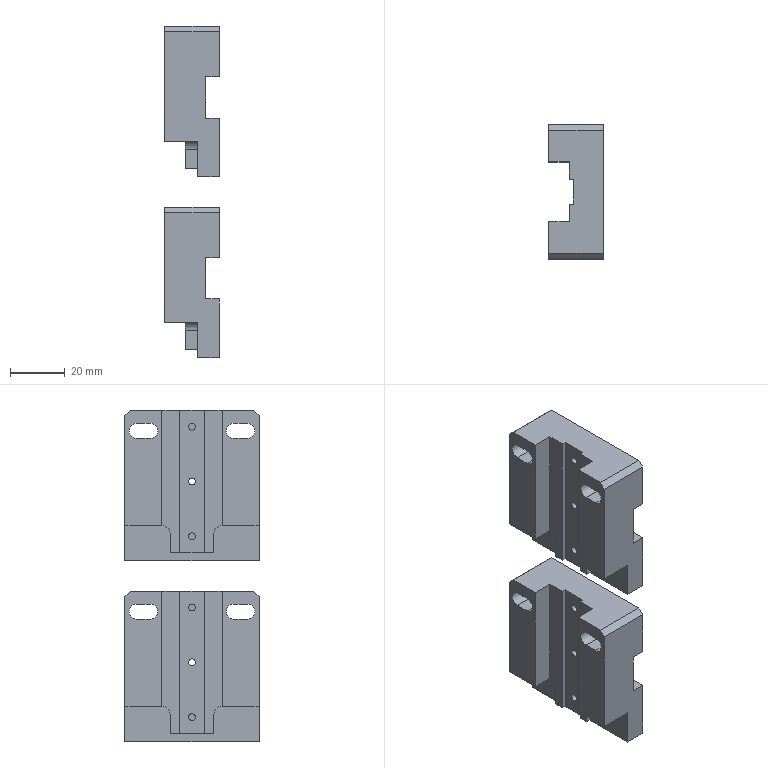CAM job | NX | 3+2 milling, drilling | part box 19.9 x 49 x 121 mm | stock box 25 x 50 x 125 mm
Tools:
number,name,description,diameter,corner_radius,flute_length,length,flutes
4,D4,平底铣刀-粗,4.0,0.0,25.0,75.0,2
6,D6,平底铣刀-粗,6.0,0.0,25.0,75.0,2
9,D10,平底铣刀-粗,10.0,0.0,35.0,75.0,2
11,D4-J,平底铣刀-精,4.0,0.0,50.0,75.0,2
7,D6-J,平底铣刀-精,6.0,0.0,25.0,75.0,2
10,D10-J,平底铣刀-精,10.0,0.0,35.0,75.0,2
1,D80R0.8飞刀,圆鼻刀-粗,80.0,0.8,50.0,75.0,2
1,D80R0.8飞刀-J,圆鼻刀-精,80.0,0.8,50.0,75.0,2
2,D6倒角刀,倒角刀,6.0,0.0,3.0,25.0,2
20,M3X0.5,丝锥,2.5,0.0,35.0,50.0,2
15,ZT5,钻头,5.0,0.0,35.0,50.0,2
12,钻头2.5,Twist Drill 2.5 mm,2.5,0.0,30.0,32.0,2
Operations:
program,operation,operation_type,tool,method,geometry_group,spindle_rpm,surface_speed,feed_per_tooth,feed_cut,feed_plunge,cut_length_mm,path_length_mm,cut_time_min,machine_time_min
B,底壁铣飞面一刀开粗_COPY,VolumeBased25DMillingOperation,D80R0.8飞刀,分层开粗-切深K-步距G,W-B,2800.0,703.696,0.5357,3000.0,100.0,2291.94,4547.238,0.764,0.9895
B,底壁铣飞面一刀精光_COPY,VolumeBased25DMillingOperation,D80R0.8飞刀-J,侧刃精光-切深K-步距G,W-B,4000.0,1005.28,0.125,1000.0,100.0,228.998,264.998,0.229,0.2326
B,底壁铣分层开粗-中_COPY,VolumeBased25DMillingOperation,D10,分层开粗-切深K-步距G,W-B,8000.0,251.32,0.25,4000.0,100.0,9132.562,9316.533,2.283,2.301
B,底壁铣分层开粗-中_COPY_1,VolumeBased25DMillingOperation,D10,分层开粗-切深K-步距G,W-B,8000.0,251.32,0.25,4000.0,100.0,9050.012,9093.878,2.263,2.267
B,底壁铣分层开粗-中_COPY_2,VolumeBased25DMillingOperation,D6,分层开粗-切深K-步距G,W-B,8000.0,150.792,0.1875,3000.0,100.0,788.28,969.914,0.2628,0.2809
B,等高光顺清角D6参考12_COPY,ZLevelMilling,D6,分层精光-切深K-步距G,W-B,8000.0,150.796,0.125,2000.0,100.0,763.584,1053.566,0.3818,0.4108
B,打点-深0.8_2,Operation,D6倒角刀,NONE,W-B,8000.0,150.796,0.0312,500.0,90.0,7.2,181.444,0.0144,0.0318
B,盲平孔-M3螺纹底孔,Operation,钻头2.5,NONE,W-B,3000.0,23.562,0.0333,200.0,90.0,36.0,239.044,0.18,0.2003
B,钻倒角_2,Operation,D6倒角刀,METHOD,W-B,8000.0,150.796,0.0312,500.0,0.0,28.5,237.067,0.057,0.0779
B,盲平孔-攻牙M3,Operation,M3X0.5,METHOD,W-B,800.0,6.283,0.0003,0.5,90.0,28.0,223.044,56.0,56.02
B,平面去毛刺6X45L_COPY,SurfaceContour,D6倒角刀,爬面_倒角-切深0-步距G,W-B,6500.0,122.519,0.1154,1500.0,100.0,1155.541,2202.729,0.7704,0.8751
B,底壁铣精光底面-中_COPY,VolumeBased25DMillingOperation,D6-J,精光步距切深关,W-B,8000.0,150.792,0.0625,1000.0,100.0,702.976,864.43,0.703,0.7191
B,底壁铣精光侧面-中-选底面_COPY,VolumeBased25DMillingOperation,D6-J,侧刃精光-切深K-步距G,W-B,8000.0,150.792,0.0625,1000.0,100.0,256.678,401.191,0.2567,0.2711
B,底壁铣精光底面-中_COPY_1,VolumeBased25DMillingOperation,D6-J,精光步距切深关,W-B,8000.0,150.792,0.0625,1000.0,100.0,412.05,572.254,0.4121,0.4281
B,底壁铣精光侧面-中-选底面_COPY_2,VolumeBased25DMillingOperation,D6-J,侧刃精光-切深K-步距G,W-B,8000.0,150.792,0.0625,1000.0,100.0,253.278,387.083,0.2533,0.2667
B,底壁铣精光侧面-中-选底面_COPY_1,VolumeBased25DMillingOperation,D6-J,侧刃精光-切深K-步距G,W-B,8000.0,150.792,0.0625,1000.0,100.0,162.338,353.415,0.1623,0.1814
A,顶面,FaceMilling,D80R0.8飞刀,侧刃精光-切深K-步距G,W-A,5000.0,1256.637,0.1,1000.0,100.0,215.0,251.0,0.215,0.2186
A,外形粗_2,VolumeBased25DMillingOperation,D10,METHOD,W-A,8000.0,251.327,0.3125,5000.0,80.0,13314.33,13497.63,2.663,2.681
A,底壁粗_1,VolumeBased25DMillingOperation,D10,METHOD,W-A,6000.0,113.0,0.2083,3500.0,100.0,2408.0,2716.48,0.688,0.7188
A,打点-深0.8,Operation,D6倒角刀,NONE,W-A,8000.0,150.796,0.0312,500.0,90.0,3.6,124.008,0.0072,0.0192
A,打点,Operation,D6倒角刀,METHOD,W-A,3000.0,56.0,0.0333,200.0,0.0,20.4,556.937,0.102,0.1557
A,预钻孔5,Operation,ZT5,METHOD,W-A,3000.0,47.124,0.0417,250.0,0.0,208.0,932.137,0.832,0.9044
A,通孔-M3螺纹底孔,Operation,钻头2.5,NONE,W-A,3000.0,23.562,0.05,300.0,90.0,25.502,167.812,0.085,0.0992
A,通腰槽粗_1,VolumeBased25DMillingOperation,D4,METHOD,W-A,6000.0,75.398,0.1,1200.0,100.0,4795.322,5168.948,3.996,4.034
A,仅选体,SurfaceContour,D6倒角刀,METHOD,W-A,8000.0,150.796,0.1875,3000.0,100.0,835.65,1745.386,0.2785,0.3695
A,钻倒角_1,Operation,D6倒角刀,METHOD,W-A,8000.0,150.796,0.0312,500.0,0.0,9.5,137.868,0.019,0.0318
A,通孔-攻牙M3,Operation,M3X0.5,METHOD,W-A,800.0,6.283,0.0003,0.5,90.0,20.0,156.808,40.0,40.014
A,底精_1,VolumeBased25DMillingOperation,D6-J,METHOD,W-A,6000.0,113.0,0.2083,1200.0,100.0,472.198,627.299,0.3935,0.409
A,底侧精_3,VolumeBased25DMillingOperation,D6-J,METHOD,W-A,6000.0,113.0,0.2083,1200.0,100.0,234.966,516.826,0.1958,0.224
A,腰槽精_1,VolumeBased25DMillingOperation,D4-J,METHOD,W-A,6000.0,113.0,0.0417,500.0,100.0,338.814,957.394,0.6776,0.7395
A,外形半精_2,VolumeBased25DMillingOperation,D10-J,METHOD,W-A,8000.0,251.327,0.0625,1000.0,100.0,977.209,1294.822,0.9772,1.009